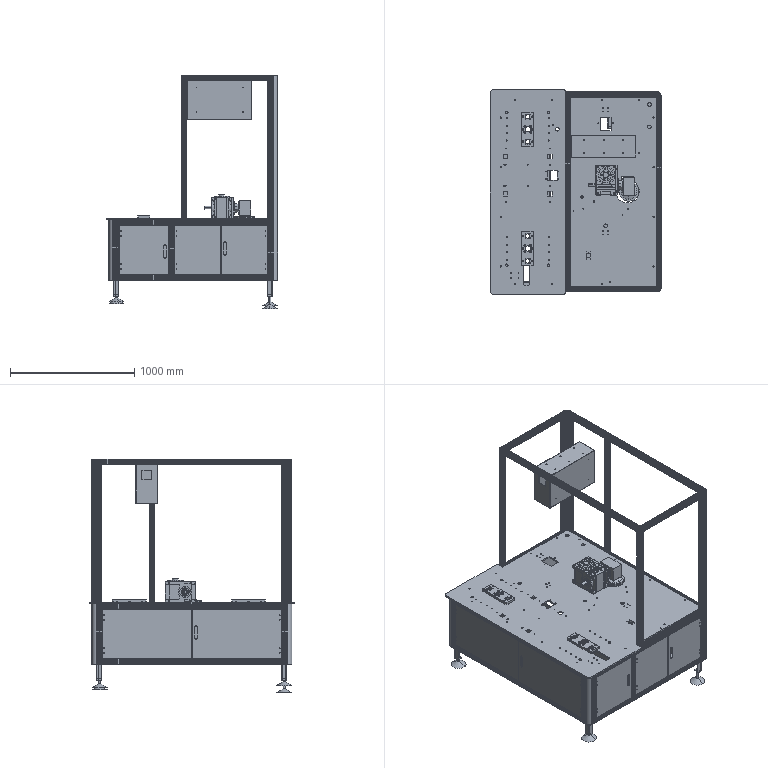Part | 101 solids | 6392 faces | volume 70429249 mm3 | plane 4180 | cylinder 1753 | spline 355 | cone 82 | torus 22 | commonest cylinder face diameters 6.8 x264 9 x214 7 x141 8.2 x134 1.473 x118 3.873 x118